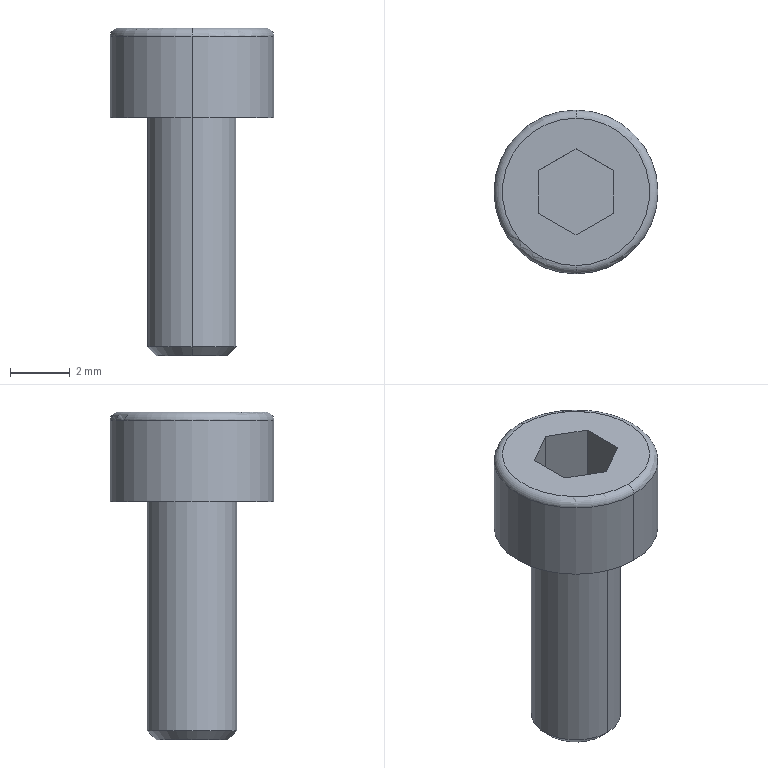Part | SolidWorks | features Chamfer 1, Fillet 1, ICE 1, Revolution 1 | 1 solid | 18 faces | box 5.5 x 5.5 x 11 mm | volume 116.734 mm3 | plane 10 | cylinder 4 | cone 2 | torus 2 | commonest cylinder face diameters 3 x2 5.5 x2
STEP:
#1=CARTESIAN_POINT('',(0.,1.2,-8.));
#2=VERTEX_POINT('',#1);
#3=CARTESIAN_POINT('',(0.,-1.2,-8.));
#4=VERTEX_POINT('',#3);
#5=CARTESIAN_POINT('',(0.,0.,-8.));
#6=DIRECTION('',(0.,0.,-1.));
#7=DIRECTION('',(0.,-1.,0.));
#8=AXIS2_PLACEMENT_3D('',#5,#6,#7);
#9=CIRCLE('',#8,1.2);
#10=EDGE_CURVE('',#2,#4,#9,.T.);
#11=ORIENTED_EDGE('',*,*,#10,.F.);
#12=CARTESIAN_POINT('',(0.,1.5,-7.7));
#13=VERTEX_POINT('',#12);
#14=CARTESIAN_POINT('',(0.,1.5,-7.7));
#15=DIRECTION('',(0.,0.7071,0.7071));
#16=VECTOR('',#15,1000.);
#17=LINE('',#14,#16);
#18=EDGE_CURVE('',#2,#13,#17,.T.);
#19=ORIENTED_EDGE('',*,*,#18,.T.);
#20=CARTESIAN_POINT('',(0.,-1.5,-7.7));
#21=VERTEX_POINT('',#20);
#22=CARTESIAN_POINT('',(0.,0.,-7.7));
#23=DIRECTION('',(0.,0.,1.));
#24=DIRECTION('',(0.,-1.,0.));
#25=AXIS2_PLACEMENT_3D('',#22,#23,#24);
#26=CIRCLE('',#25,1.5);
#27=EDGE_CURVE('',#21,#13,#26,.T.);
#28=ORIENTED_EDGE('',*,*,#27,.F.);
#29=CARTESIAN_POINT('',(0.,-1.5,-7.7));
#30=DIRECTION('',(0.,-0.7071,0.7071));
#31=VECTOR('',#30,1000.);
#32=LINE('',#29,#31);
#33=EDGE_CURVE('',#4,#21,#32,.T.);
#34=ORIENTED_EDGE('',*,*,#33,.F.);
#35=EDGE_LOOP('',(#11,#19,#28,#34));
#36=FACE_OUTER_BOUND('',#35,.T.);
#37=CARTESIAN_POINT('',(0.,0.,-7.7));
#38=DIRECTION('',(0.,0.,1.));
#39=DIRECTION('',(0.,-1.,0.));
#40=AXIS2_PLACEMENT_3D('',#37,#38,#39);
#41=CONICAL_SURFACE('',#40,1.5,0.7854);
#42=ADVANCED_FACE('',(#36),#41,.T.);
#43=CARTESIAN_POINT('',(0.,-2.475,3.));
#44=VERTEX_POINT('',#43);
#45=CARTESIAN_POINT('',(0.,2.475,3.));
#46=VERTEX_POINT('',#45);
#47=CARTESIAN_POINT('',(0.,0.,3.));
#48=DIRECTION('',(0.,0.,1.));
#49=DIRECTION('',(0.,1.,0.));
#50=AXIS2_PLACEMENT_3D('',#47,#48,#49);
#51=CIRCLE('',#50,2.475);
#52=EDGE_CURVE('',#44,#46,#51,.T.);
#53=ORIENTED_EDGE('',*,*,#52,.F.);
#54=CARTESIAN_POINT('',(0.,-2.75,2.725));
#55=VERTEX_POINT('',#54);
#56=CARTESIAN_POINT('',(0.,-2.475,2.725));
#57=DIRECTION('',(1.,0.,0.));
#58=DIRECTION('',(0.,1.,0.));
#59=AXIS2_PLACEMENT_3D('',#56,#57,#58);
#60=CIRCLE('',#59,0.275);
#61=EDGE_CURVE('',#44,#55,#60,.T.);
#62=ORIENTED_EDGE('',*,*,#61,.T.);
#63=CARTESIAN_POINT('',(0.,2.75,2.725));
#64=VERTEX_POINT('',#63);
#65=CARTESIAN_POINT('',(0.,0.,2.725));
#66=DIRECTION('',(0.,0.,-1.));
#67=DIRECTION('',(0.,1.,0.));
#68=AXIS2_PLACEMENT_3D('',#65,#66,#67);
#69=CIRCLE('',#68,2.75);
#70=EDGE_CURVE('',#64,#55,#69,.T.);
#71=ORIENTED_EDGE('',*,*,#70,.F.);
#72=CARTESIAN_POINT('',(0.,2.475,2.725));
#73=DIRECTION('',(-1.,0.,0.));
#74=DIRECTION('',(0.,0.,1.));
#75=AXIS2_PLACEMENT_3D('',#72,#73,#74);
#76=CIRCLE('',#75,0.275);
#77=EDGE_CURVE('',#46,#64,#76,.T.);
#78=ORIENTED_EDGE('',*,*,#77,.F.);
#79=EDGE_LOOP('',(#53,#62,#71,#78));
#80=FACE_OUTER_BOUND('',#79,.T.);
#81=CARTESIAN_POINT('',(0.,0.,2.725));
#82=DIRECTION('',(0.,0.,-1.));
#83=DIRECTION('',(0.,1.,0.));
#84=AXIS2_PLACEMENT_3D('',#81,#82,#83);
#85=TOROIDAL_SURFACE('',#84,2.475,0.275);
#86=ADVANCED_FACE('',(#80),#85,.T.);
#87=ORIENTED_EDGE('',*,*,#27,.T.);
#88=CARTESIAN_POINT('',(0.,1.5,0.));
#89=VERTEX_POINT('',#88);
#90=CARTESIAN_POINT('',(0.,1.5,3.));
#91=DIRECTION('',(0.,0.,1.));
#92=VECTOR('',#91,1000.);
#93=LINE('',#90,#92);
#94=EDGE_CURVE('',#13,#89,#93,.T.);
#95=ORIENTED_EDGE('',*,*,#94,.T.);
#96=CARTESIAN_POINT('',(0.,-1.5,0.));
#97=VERTEX_POINT('',#96);
#98=CARTESIAN_POINT('',(0.,0.,0.));
#99=DIRECTION('',(0.,0.,1.));
#100=DIRECTION('',(0.,-1.,0.));
#101=AXIS2_PLACEMENT_3D('',#98,#99,#100);
#102=CIRCLE('',#101,1.5);
#103=EDGE_CURVE('',#97,#89,#102,.T.);
#104=ORIENTED_EDGE('',*,*,#103,.F.);
#105=CARTESIAN_POINT('',(0.,-1.5,3.));
#106=DIRECTION('',(0.,0.,1.));
#107=VECTOR('',#106,1000.);
#108=LINE('',#105,#107);
#109=EDGE_CURVE('',#21,#97,#108,.T.);
#110=ORIENTED_EDGE('',*,*,#109,.F.);
#111=EDGE_LOOP('',(#87,#95,#104,#110));
#112=FACE_OUTER_BOUND('',#111,.T.);
#113=CARTESIAN_POINT('',(0.,0.,3.));
#114=DIRECTION('',(0.,0.,1.));
#115=DIRECTION('',(0.,-1.,0.));
#116=AXIS2_PLACEMENT_3D('',#113,#114,#115);
#117=CYLINDRICAL_SURFACE('',#116,1.5);
#118=ADVANCED_FACE('',(#112),#117,.T.);
#119=CARTESIAN_POINT('',(0.,-2.75,0.));
#120=VERTEX_POINT('',#119);
#121=CARTESIAN_POINT('',(0.,2.75,0.));
#122=VERTEX_POINT('',#121);
#123=CARTESIAN_POINT('',(0.,0.,0.));
#124=DIRECTION('',(0.,0.,1.));
#125=DIRECTION('',(0.,-1.,0.));
#126=AXIS2_PLACEMENT_3D('',#123,#124,#125);
#127=CIRCLE('',#126,2.75);
#128=EDGE_CURVE('',#120,#122,#127,.T.);
#129=ORIENTED_EDGE('',*,*,#128,.T.);
#130=CARTESIAN_POINT('',(0.,2.75,3.));
#131=DIRECTION('',(0.,0.,1.));
#132=VECTOR('',#131,1000.);
#133=LINE('',#130,#132);
#134=EDGE_CURVE('',#122,#64,#133,.T.);
#135=ORIENTED_EDGE('',*,*,#134,.T.);
#136=ORIENTED_EDGE('',*,*,#70,.T.);
#137=CARTESIAN_POINT('',(0.,-2.75,3.));
#138=DIRECTION('',(0.,0.,1.));
#139=VECTOR('',#138,1000.);
#140=LINE('',#137,#139);
#141=EDGE_CURVE('',#120,#55,#140,.T.);
#142=ORIENTED_EDGE('',*,*,#141,.F.);
#143=EDGE_LOOP('',(#129,#135,#136,#142));
#144=FACE_OUTER_BOUND('',#143,.T.);
#145=CARTESIAN_POINT('',(0.,0.,3.));
#146=DIRECTION('',(0.,0.,1.));
#147=DIRECTION('',(0.,-1.,0.));
#148=AXIS2_PLACEMENT_3D('',#145,#146,#147);
#149=CYLINDRICAL_SURFACE('',#148,2.75);
#150=ADVANCED_FACE('',(#144),#149,.T.);
#151=CARTESIAN_POINT('',(0.,0.,3.));
#152=DIRECTION('',(0.,0.,1.));
#153=DIRECTION('',(0.,1.,0.));
#154=AXIS2_PLACEMENT_3D('',#151,#152,#153);
#155=CIRCLE('',#154,2.475);
#156=EDGE_CURVE('',#46,#44,#155,.T.);
#157=ORIENTED_EDGE('',*,*,#156,.T.);
#158=ORIENTED_EDGE('',*,*,#52,.T.);
#159=EDGE_LOOP('',(#157,#158));
#160=FACE_OUTER_BOUND('',#159,.T.);
#161=CARTESIAN_POINT('',(0.,1.443,3.));
#162=VERTEX_POINT('',#161);
#163=CARTESIAN_POINT('',(-1.25,0.7217,3.));
#164=VERTEX_POINT('',#163);
#165=CARTESIAN_POINT('',(0.,1.443,3.));
#166=DIRECTION('',(-0.866,-0.5,0.));
#167=VECTOR('',#166,1000.);
#168=LINE('',#165,#167);
#169=EDGE_CURVE('',#162,#164,#168,.T.);
#170=ORIENTED_EDGE('',*,*,#169,.F.);
#171=CARTESIAN_POINT('',(1.25,0.7217,3.));
#172=VERTEX_POINT('',#171);
#173=CARTESIAN_POINT('',(1.25,0.7217,3.));
#174=DIRECTION('',(-0.866,0.5,0.));
#175=VECTOR('',#174,1000.);
#176=LINE('',#173,#175);
#177=EDGE_CURVE('',#172,#162,#176,.T.);
#178=ORIENTED_EDGE('',*,*,#177,.F.);
#179=CARTESIAN_POINT('',(1.25,-0.7217,3.));
#180=VERTEX_POINT('',#179);
#181=CARTESIAN_POINT('',(1.25,-0.7217,3.));
#182=DIRECTION('',(0.,1.,0.));
#183=VECTOR('',#182,1000.);
#184=LINE('',#181,#183);
#185=EDGE_CURVE('',#180,#172,#184,.T.);
#186=ORIENTED_EDGE('',*,*,#185,.F.);
#187=CARTESIAN_POINT('',(0.,-1.443,3.));
#188=VERTEX_POINT('',#187);
#189=CARTESIAN_POINT('',(0.,-1.443,3.));
#190=DIRECTION('',(0.866,0.5,0.));
#191=VECTOR('',#190,1000.);
#192=LINE('',#189,#191);
#193=EDGE_CURVE('',#188,#180,#192,.T.);
#194=ORIENTED_EDGE('',*,*,#193,.F.);
#195=CARTESIAN_POINT('',(-1.25,-0.7217,3.));
#196=VERTEX_POINT('',#195);
#197=CARTESIAN_POINT('',(-1.25,-0.7217,3.));
#198=DIRECTION('',(0.866,-0.5,0.));
#199=VECTOR('',#198,1000.);
#200=LINE('',#197,#199);
#201=EDGE_CURVE('',#196,#188,#200,.T.);
#202=ORIENTED_EDGE('',*,*,#201,.F.);
#203=CARTESIAN_POINT('',(-1.25,0.7217,3.));
#204=DIRECTION('',(0.,-1.,0.));
#205=VECTOR('',#204,1000.);
#206=LINE('',#203,#205);
#207=EDGE_CURVE('',#164,#196,#206,.T.);
#208=ORIENTED_EDGE('',*,*,#207,.F.);
#209=EDGE_LOOP('',(#170,#178,#186,#194,#202,#208));
#210=FACE_BOUND('',#209,.T.);
#211=CARTESIAN_POINT('',(0.,0.,3.));
#212=DIRECTION('',(0.,0.,-1.));
#213=DIRECTION('',(0.,1.,0.));
#214=AXIS2_PLACEMENT_3D('',#211,#212,#213);
#215=PLANE('',#214);
#216=ADVANCED_FACE('',(#160,#210),#215,.F.);
#217=ORIENTED_EDGE('',*,*,#134,.F.);
#218=CARTESIAN_POINT('',(0.,0.,0.));
#219=DIRECTION('',(0.,0.,1.));
#220=DIRECTION('',(0.,-1.,0.));
#221=AXIS2_PLACEMENT_3D('',#218,#219,#220);
#222=CIRCLE('',#221,2.75);
#223=EDGE_CURVE('',#122,#120,#222,.T.);
#224=ORIENTED_EDGE('',*,*,#223,.T.);
#225=ORIENTED_EDGE('',*,*,#141,.T.);
#226=CARTESIAN_POINT('',(0.,0.,2.725));
#227=DIRECTION('',(0.,0.,-1.));
#228=DIRECTION('',(0.,1.,0.));
#229=AXIS2_PLACEMENT_3D('',#226,#227,#228);
#230=CIRCLE('',#229,2.75);
#231=EDGE_CURVE('',#55,#64,#230,.T.);
#232=ORIENTED_EDGE('',*,*,#231,.T.);
#233=EDGE_LOOP('',(#217,#224,#225,#232));
#234=FACE_OUTER_BOUND('',#233,.T.);
#235=CARTESIAN_POINT('',(0.,0.,3.));
#236=DIRECTION('',(0.,0.,1.));
#237=DIRECTION('',(0.,-1.,0.));
#238=AXIS2_PLACEMENT_3D('',#235,#236,#237);
#239=CYLINDRICAL_SURFACE('',#238,2.75);
#240=ADVANCED_FACE('',(#234),#239,.T.);
#241=ORIENTED_EDGE('',*,*,#128,.F.);
#242=ORIENTED_EDGE('',*,*,#223,.F.);
#243=EDGE_LOOP('',(#241,#242));
#244=FACE_OUTER_BOUND('',#243,.T.);
#245=ORIENTED_EDGE('',*,*,#103,.T.);
#246=CARTESIAN_POINT('',(0.,0.,0.));
#247=DIRECTION('',(0.,0.,1.));
#248=DIRECTION('',(0.,-1.,0.));
#249=AXIS2_PLACEMENT_3D('',#246,#247,#248);
#250=CIRCLE('',#249,1.5);
#251=EDGE_CURVE('',#89,#97,#250,.T.);
#252=ORIENTED_EDGE('',*,*,#251,.T.);
#253=EDGE_LOOP('',(#245,#252));
#254=FACE_BOUND('',#253,.T.);
#255=CARTESIAN_POINT('',(0.,2.75,0.));
#256=DIRECTION('',(0.,0.,1.));
#257=DIRECTION('',(0.,-1.,0.));
#258=AXIS2_PLACEMENT_3D('',#255,#256,#257);
#259=PLANE('',#258);
#260=ADVANCED_FACE('',(#244,#254),#259,.F.);
#261=ORIENTED_EDGE('',*,*,#94,.F.);
#262=CARTESIAN_POINT('',(0.,0.,-7.7));
#263=DIRECTION('',(0.,0.,1.));
#264=DIRECTION('',(0.,-1.,0.));
#265=AXIS2_PLACEMENT_3D('',#262,#263,#264);
#266=CIRCLE('',#265,1.5);
#267=EDGE_CURVE('',#13,#21,#266,.T.);
#268=ORIENTED_EDGE('',*,*,#267,.T.);
#269=ORIENTED_EDGE('',*,*,#109,.T.);
#270=ORIENTED_EDGE('',*,*,#251,.F.);
#271=EDGE_LOOP('',(#261,#268,#269,#270));
#272=FACE_OUTER_BOUND('',#271,.T.);
#273=CARTESIAN_POINT('',(0.,0.,3.));
#274=DIRECTION('',(0.,0.,1.));
#275=DIRECTION('',(0.,-1.,0.));
#276=AXIS2_PLACEMENT_3D('',#273,#274,#275);
#277=CYLINDRICAL_SURFACE('',#276,1.5);
#278=ADVANCED_FACE('',(#272),#277,.T.);
#279=CARTESIAN_POINT('',(0.,0.,-8.));
#280=DIRECTION('',(0.,0.,-1.));
#281=DIRECTION('',(0.,-1.,0.));
#282=AXIS2_PLACEMENT_3D('',#279,#280,#281);
#283=CIRCLE('',#282,1.2);
#284=EDGE_CURVE('',#4,#2,#283,.T.);
#285=ORIENTED_EDGE('',*,*,#284,.T.);
#286=ORIENTED_EDGE('',*,*,#10,.T.);
#287=EDGE_LOOP('',(#285,#286));
#288=FACE_OUTER_BOUND('',#287,.T.);
#289=CARTESIAN_POINT('',(0.,1.5,-8.));
#290=DIRECTION('',(0.,0.,1.));
#291=DIRECTION('',(0.,-1.,0.));
#292=AXIS2_PLACEMENT_3D('',#289,#290,#291);
#293=PLANE('',#292);
#294=ADVANCED_FACE('',(#288),#293,.F.);
#295=ORIENTED_EDGE('',*,*,#177,.T.);
#296=CARTESIAN_POINT('',(0.,1.443,1.075));
#297=VERTEX_POINT('',#296);
#298=CARTESIAN_POINT('',(0.,1.443,1.075));
#299=DIRECTION('',(0.,0.,1.));
#300=VECTOR('',#299,1000.);
#301=LINE('',#298,#300);
#302=EDGE_CURVE('',#297,#162,#301,.T.);
#303=ORIENTED_EDGE('',*,*,#302,.F.);
#304=CARTESIAN_POINT('',(1.25,0.7217,1.075));
#305=VERTEX_POINT('',#304);
#306=CARTESIAN_POINT('',(1.25,0.7217,1.075));
#307=DIRECTION('',(-0.866,0.5,0.));
#308=VECTOR('',#307,1000.);
#309=LINE('',#306,#308);
#310=EDGE_CURVE('',#305,#297,#309,.T.);
#311=ORIENTED_EDGE('',*,*,#310,.F.);
#312=CARTESIAN_POINT('',(1.25,0.7217,1.075));
#313=DIRECTION('',(0.,0.,1.));
#314=VECTOR('',#313,1000.);
#315=LINE('',#312,#314);
#316=EDGE_CURVE('',#305,#172,#315,.T.);
#317=ORIENTED_EDGE('',*,*,#316,.T.);
#318=EDGE_LOOP('',(#295,#303,#311,#317));
#319=FACE_OUTER_BOUND('',#318,.T.);
#320=CARTESIAN_POINT('',(1.25,0.7217,1.075));
#321=DIRECTION('',(0.5,0.866,0.));
#322=DIRECTION('',(-0.866,0.5,0.));
#323=AXIS2_PLACEMENT_3D('',#320,#321,#322);
#324=PLANE('',#323);
#325=ADVANCED_FACE('',(#319),#324,.F.);
#326=ORIENTED_EDGE('',*,*,#185,.T.);
#327=ORIENTED_EDGE('',*,*,#316,.F.);
#328=CARTESIAN_POINT('',(1.25,-0.7217,1.075));
#329=VERTEX_POINT('',#328);
#330=CARTESIAN_POINT('',(1.25,-0.7217,1.075));
#331=DIRECTION('',(0.,1.,0.));
#332=VECTOR('',#331,1000.);
#333=LINE('',#330,#332);
#334=EDGE_CURVE('',#329,#305,#333,.T.);
#335=ORIENTED_EDGE('',*,*,#334,.F.);
#336=CARTESIAN_POINT('',(1.25,-0.7217,1.075));
#337=DIRECTION('',(0.,0.,1.));
#338=VECTOR('',#337,1000.);
#339=LINE('',#336,#338);
#340=EDGE_CURVE('',#329,#180,#339,.T.);
#341=ORIENTED_EDGE('',*,*,#340,.T.);
#342=EDGE_LOOP('',(#326,#327,#335,#341));
#343=FACE_OUTER_BOUND('',#342,.T.);
#344=CARTESIAN_POINT('',(1.25,-0.7217,1.075));
#345=DIRECTION('',(1.,0.,0.));
#346=DIRECTION('',(0.,0.,-1.));
#347=AXIS2_PLACEMENT_3D('',#344,#345,#346);
#348=PLANE('',#347);
#349=ADVANCED_FACE('',(#343),#348,.F.);
#350=ORIENTED_EDGE('',*,*,#193,.T.);
#351=ORIENTED_EDGE('',*,*,#340,.F.);
#352=CARTESIAN_POINT('',(0.,-1.443,1.075));
#353=VERTEX_POINT('',#352);
#354=CARTESIAN_POINT('',(0.,-1.443,1.075));
#355=DIRECTION('',(0.866,0.5,0.));
#356=VECTOR('',#355,1000.);
#357=LINE('',#354,#356);
#358=EDGE_CURVE('',#353,#329,#357,.T.);
#359=ORIENTED_EDGE('',*,*,#358,.F.);
#360=CARTESIAN_POINT('',(0.,-1.443,1.075));
#361=DIRECTION('',(0.,0.,1.));
#362=VECTOR('',#361,1000.);
#363=LINE('',#360,#362);
#364=EDGE_CURVE('',#353,#188,#363,.T.);
#365=ORIENTED_EDGE('',*,*,#364,.T.);
#366=EDGE_LOOP('',(#350,#351,#359,#365));
#367=FACE_OUTER_BOUND('',#366,.T.);
#368=CARTESIAN_POINT('',(0.,-1.443,1.075));
#369=DIRECTION('',(0.5,-0.866,0.));
#370=DIRECTION('',(0.866,0.5,0.));
#371=AXIS2_PLACEMENT_3D('',#368,#369,#370);
#372=PLANE('',#371);
#373=ADVANCED_FACE('',(#367),#372,.F.);
#374=ORIENTED_EDGE('',*,*,#201,.T.);
#375=ORIENTED_EDGE('',*,*,#364,.F.);
#376=CARTESIAN_POINT('',(-1.25,-0.7217,1.075));
#377=VERTEX_POINT('',#376);
#378=CARTESIAN_POINT('',(-1.25,-0.7217,1.075));
#379=DIRECTION('',(0.866,-0.5,0.));
#380=VECTOR('',#379,1000.);
#381=LINE('',#378,#380);
#382=EDGE_CURVE('',#377,#353,#381,.T.);
#383=ORIENTED_EDGE('',*,*,#382,.F.);
#384=CARTESIAN_POINT('',(-1.25,-0.7217,1.075));
#385=DIRECTION('',(0.,0.,1.));
#386=VECTOR('',#385,1000.);
#387=LINE('',#384,#386);
#388=EDGE_CURVE('',#377,#196,#387,.T.);
#389=ORIENTED_EDGE('',*,*,#388,.T.);
#390=EDGE_LOOP('',(#374,#375,#383,#389));
#391=FACE_OUTER_BOUND('',#390,.T.);
#392=CARTESIAN_POINT('',(-1.25,-0.7217,1.075));
#393=DIRECTION('',(-0.5,-0.866,0.));
#394=DIRECTION('',(0.866,-0.5,0.));
#395=AXIS2_PLACEMENT_3D('',#392,#393,#394);
#396=PLANE('',#395);
#397=ADVANCED_FACE('',(#391),#396,.F.);
#398=ORIENTED_EDGE('',*,*,#207,.T.);
#399=ORIENTED_EDGE('',*,*,#388,.F.);
#400=CARTESIAN_POINT('',(-1.25,0.7217,1.075));
#401=VERTEX_POINT('',#400);
#402=CARTESIAN_POINT('',(-1.25,0.7217,1.075));
#403=DIRECTION('',(0.,-1.,0.));
#404=VECTOR('',#403,1000.);
#405=LINE('',#402,#404);
#406=EDGE_CURVE('',#401,#377,#405,.T.);
#407=ORIENTED_EDGE('',*,*,#406,.F.);
#408=CARTESIAN_POINT('',(-1.25,0.7217,1.075));
#409=DIRECTION('',(0.,0.,1.));
#410=VECTOR('',#409,1000.);
#411=LINE('',#408,#410);
#412=EDGE_CURVE('',#401,#164,#411,.T.);
#413=ORIENTED_EDGE('',*,*,#412,.T.);
#414=EDGE_LOOP('',(#398,#399,#407,#413));
#415=FACE_OUTER_BOUND('',#414,.T.);
#416=CARTESIAN_POINT('',(-1.25,0.7217,1.075));
#417=DIRECTION('',(-1.,0.,0.));
#418=DIRECTION('',(0.,-1.,0.));
#419=AXIS2_PLACEMENT_3D('',#416,#417,#418);
#420=PLANE('',#419);
#421=ADVANCED_FACE('',(#415),#420,.F.);
#422=ORIENTED_EDGE('',*,*,#169,.T.);
#423=ORIENTED_EDGE('',*,*,#412,.F.);
#424=CARTESIAN_POINT('',(0.,1.443,1.075));
#425=DIRECTION('',(-0.866,-0.5,0.));
#426=VECTOR('',#425,1000.);
#427=LINE('',#424,#426);
#428=EDGE_CURVE('',#297,#401,#427,.T.);
#429=ORIENTED_EDGE('',*,*,#428,.F.);
#430=ORIENTED_EDGE('',*,*,#302,.T.);
#431=EDGE_LOOP('',(#422,#423,#429,#430));
#432=FACE_OUTER_BOUND('',#431,.T.);
#433=CARTESIAN_POINT('',(0.,1.443,1.075));
#434=DIRECTION('',(-0.5,0.866,0.));
#435=DIRECTION('',(-0.866,-0.5,0.));
#436=AXIS2_PLACEMENT_3D('',#433,#434,#435);
#437=PLANE('',#436);
#438=ADVANCED_FACE('',(#432),#437,.F.);
#439=ORIENTED_EDGE('',*,*,#310,.T.);
#440=ORIENTED_EDGE('',*,*,#428,.T.);
#441=ORIENTED_EDGE('',*,*,#406,.T.);
#442=ORIENTED_EDGE('',*,*,#382,.T.);
#443=ORIENTED_EDGE('',*,*,#358,.T.);
#444=ORIENTED_EDGE('',*,*,#334,.T.);
#445=EDGE_LOOP('',(#439,#440,#441,#442,#443,#444));
#446=FACE_OUTER_BOUND('',#445,.T.);
#447=CARTESIAN_POINT('',(0.,1.443,1.075));
#448=DIRECTION('',(0.,0.,1.));
#449=DIRECTION('',(1.,0.,0.));
#450=AXIS2_PLACEMENT_3D('',#447,#448,#449);
#451=PLANE('',#450);
#452=ADVANCED_FACE('',(#446),#451,.T.);
#453=ORIENTED_EDGE('',*,*,#61,.F.);
#454=ORIENTED_EDGE('',*,*,#156,.F.);
#455=ORIENTED_EDGE('',*,*,#77,.T.);
#456=ORIENTED_EDGE('',*,*,#231,.F.);
#457=EDGE_LOOP('',(#453,#454,#455,#456));
#458=FACE_OUTER_BOUND('',#457,.T.);
#459=CARTESIAN_POINT('',(0.,0.,2.725));
#460=DIRECTION('',(0.,0.,-1.));
#461=DIRECTION('',(0.,1.,0.));
#462=AXIS2_PLACEMENT_3D('',#459,#460,#461);
#463=TOROIDAL_SURFACE('',#462,2.475,0.275);
#464=ADVANCED_FACE('',(#458),#463,.T.);
#465=ORIENTED_EDGE('',*,*,#18,.F.);
#466=ORIENTED_EDGE('',*,*,#284,.F.);
#467=ORIENTED_EDGE('',*,*,#33,.T.);
#468=ORIENTED_EDGE('',*,*,#267,.F.);
#469=EDGE_LOOP('',(#465,#466,#467,#468));
#470=FACE_OUTER_BOUND('',#469,.T.);
#471=CARTESIAN_POINT('',(0.,0.,-7.7));
#472=DIRECTION('',(0.,0.,1.));
#473=DIRECTION('',(0.,-1.,0.));
#474=AXIS2_PLACEMENT_3D('',#471,#472,#473);
#475=CONICAL_SURFACE('',#474,1.5,0.7854);
#476=ADVANCED_FACE('',(#470),#475,.T.);
#477=CLOSED_SHELL('',(#42,#86,#118,#150,#216,#240,#260,#278,#294,#325,#349,#373,#397,#421,#438,#452,#464,#476));
#478=MANIFOLD_SOLID_BREP('',#477);
#479=CARTESIAN_POINT('',(0.,0.,0.));
#480=DIRECTION('',(0.,0.,1.));
#481=DIRECTION('',(1.,0.,0.));
#482=AXIS2_PLACEMENT_3D('',#479,#480,#481);
#483=(LENGTH_UNIT()NAMED_UNIT(*)SI_UNIT(.MILLI.,.METRE.));
#484=UNCERTAINTY_MEASURE_WITH_UNIT(LENGTH_MEASURE(0.00001),#483,'','');
#485=(NAMED_UNIT(*)PLANE_ANGLE_UNIT()SI_UNIT($,.RADIAN.));
#486=(NAMED_UNIT(*)SI_UNIT($,.STERADIAN.)SOLID_ANGLE_UNIT());
#487=(GEOMETRIC_REPRESENTATION_CONTEXT(3)GLOBAL_UNCERTAINTY_ASSIGNED_CONTEXT((#484))GLOBAL_UNIT_ASSIGNED_CONTEXT((#483,#485,#486))REPRESENTATION_CONTEXT('',''));
#488=ADVANCED_BREP_SHAPE_REPRESENTATION('',(#478,#482),#487);